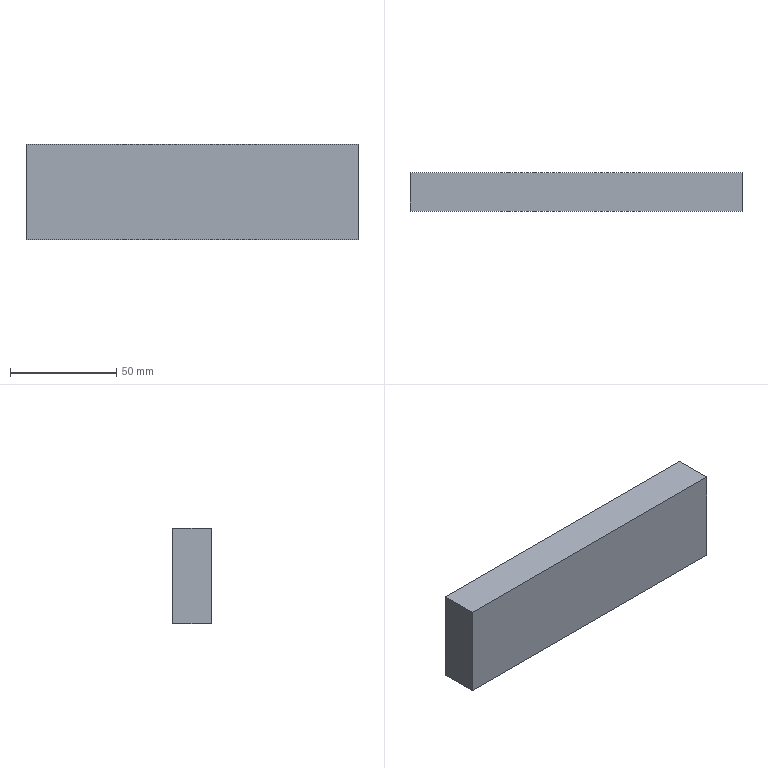NC program | NX | posted with a generic post | part box 156 x 18 x 45 mm
Lines 2243 to 3545 of 3545:
(FLOOR_WALL , TOOL : D4C)
N4424 T03 M6
N4426 G53
N4428 G17 G0 G90 X-18.397 Y-4.1 S3500 M3
N4430 G43 Z19.87 H3
N4432 Z1.825
N4434 G94 G1 Z-0.175 F1500.
N4436 Y-2.
N4438 Y42.
N4440 X-17.1
N4442 Y-2.
N4444 Y-4.1
N4446 Z1.825
N4448 G0 X-18.397 Z1.63
N4450 G1 Z-0.37
N4452 Y-2.
N4454 Y42.
N4456 X-17.1
N4458 Y-2.
N4460 Y-4.1
N4462 Z1.63
N4464 G0 X-18.397 Z1.434
N4466 G1 Z-0.566
N4468 Y-2.
N4470 Y42.
N4472 X-17.1
N4474 Y-2.
N4476 Y-4.1
N4478 Z1.434
N4480 G0 X-18.397 Z1.239
N4482 G1 Z-0.761
N4484 Y-2.
N4486 Y42.
N4488 X-17.1
N4490 Y-2.
N4492 Y-4.1
N4494 Z1.239
N4496 G0 X-18.397 Z1.044
N4498 G1 Z-0.956
N4500 Y-2.
N4502 Y42.
N4504 X-17.1
N4506 Y-2.
N4508 Y-4.1
N4510 Z1.044
N4512 G0 X-18.397 Z0.849
N4514 G1 Z-1.151
N4516 Y-2.
N4518 Y42.
N4520 X-17.1
N4522 Y-2.
N4524 Y-4.1
N4526 Z0.849
N4528 G0 X-18.397 Z0.653
N4530 G1 Z-1.347
N4532 Y-2.
N4534 Y42.
N4536 X-17.1
N4538 Y-2.
N4540 Y-4.1
N4542 Z0.653
N4544 G0 X-18.397 Z0.458
N4546 G1 Z-1.542
N4548 Y-2.
N4550 Y42.
N4552 X-17.1
N4554 Y-2.
N4556 Y-4.1
N4558 Z0.458
N4560 G0 X-18.397 Z0.263
N4562 G1 Z-1.737
N4564 Y-2.
N4566 Y42.
N4568 X-17.1
N4570 Y-2.
N4572 Y-4.1
N4574 Z0.263
N4576 G0 X-18.397 Z0.068
N4578 G1 Z-1.932
N4580 Y-2.
N4582 Y42.
N4584 X-17.1
N4586 Y-2.
N4588 Y-4.1
N4590 Z0.068
N4592 G0 X-18.397 Z-0.128
N4594 G1 Z-2.128
N4596 Y-2.
N4598 Y42.
N4600 X-17.1
N4602 Y-2.
N4604 Y-4.1
N4606 Z-0.128
N4608 G0 X-18.397 Z-0.323
N4610 G1 Z-2.323
N4612 Y-2.
N4614 Y42.
N4616 X-17.1
N4618 Y-2.
N4620 Y-4.1
N4622 Z-0.323
N4624 G0 X-18.397 Z-0.518
N4626 G1 Z-2.518
N4628 Y-2.
N4630 Y42.
N4632 X-17.1
N4634 Y-2.
N4636 Y-4.1
N4638 Z-0.518
N4640 G0 X-18.397 Z-0.713
N4642 G1 Z-2.713
N4644 Y-2.
N4646 Y42.
N4648 X-17.1
N4650 Y-2.
N4652 Y-4.1
N4654 Z-0.713
N4656 G0 X-18.397 Z-0.909
N4658 G1 Z-2.909
N4660 Y-2.
N4662 Y42.
N4664 X-17.1
N4666 Y-2.
N4668 Y-4.1
N4670 Z-0.909
N4672 G0 X-18.397 Z-1.104
N4674 G1 Z-3.104
N4676 Y-2.
N4678 Y42.
N4680 X-17.1
N4682 Y-2.
N4684 Y-4.1
N4686 Z-1.104
N4688 G0 X-18.397 Z-1.299
N4690 G1 Z-3.299
N4692 Y-2.
N4694 Y42.
N4696 X-17.1
N4698 Y-2.
N4700 Y-4.1
N4702 Z-1.299
N4704 G0 X-18.397 Z-1.494
N4706 G1 Z-3.494
N4708 Y-2.
N4710 Y42.
N4712 X-17.1
N4714 Y-2.
N4716 Y-4.1
N4718 Z-1.494
N4720 G0 X-18.397 Z-1.69
N4722 G1 Z-3.69
N4724 Y-2.
N4726 Y42.
N4728 X-17.1
N4730 Y-2.
N4732 Y-4.1
N4734 Z-1.69
N4736 G0 X-18.397 Z-1.885
N4738 G1 Z-3.885
N4740 Y-2.
N4742 Y42.
N4744 X-17.1
N4746 Y-2.
N4748 Y-4.1
N4750 Z-1.885
N4752 G0 X-18.397 Z-2.08
N4754 G1 Z-4.08
N4756 Y-2.
N4758 Y42.
N4760 X-17.1
N4762 Y-2.
N4764 Y-4.1
N4766 Z-2.08
N4768 G0 Z19.87
(PLANAR_MILL_4 , TOOL : D4C)
N4770 X-6.35 Y28.212
N4772 Z0.37
N4774 G1 Y33.264 Z0.357
N4776 X-6.666 Y33.834 Z0.355
N4778 X-7.236 Y34.15 Z0.353
N4780 X-7.764 Z0.352
N4782 X-8.334 Y33.834 Z0.35
N4784 X-8.65 Y33.264 Z0.349
N4786 Y6.736 Z0.279
N4788 X-8.334 Y6.166 Z0.277
N4790 X-7.764 Y5.85 Z0.276
N4792 X-7.236 Z0.274
N4794 X-6.666 Y6.166 Z0.273
N4796 X-6.35 Y6.736 Z0.271
N4798 Y33.264 Z0.201
N4800 X-6.666 Y33.834 Z0.2
N4802 X-7.236 Y34.15 Z0.198
N4804 X-7.764 Z0.197
N4806 X-8.334 Y33.834 Z0.195
N4808 X-8.65 Y33.264 Z0.193
N4810 Y6.736 Z0.124
N4812 X-8.334 Y6.166 Z0.122
N4814 X-7.764 Y5.85 Z0.12
N4816 X-7.236 Z0.119
N4818 X-6.666 Y6.166 Z0.117
N4820 X-6.35 Y6.736 Z0.116
N4822 Y33.264 Z0.046
N4824 X-6.666 Y33.834 Z0.044
N4826 X-7.236 Y34.15 Z0.043
N4828 X-7.764 Z0.041
N4830 X-8.334 Y33.834 Z0.04
N4832 X-8.65 Y33.264 Z0.038
N4834 Y6.736 Z-0.032
N4836 X-8.334 Y6.166 Z-0.033
N4838 X-7.764 Y5.85 Z-0.035
N4840 X-7.236 Z-0.036
N4842 X-6.666 Y6.166 Z-0.038
N4844 X-6.35 Y6.736 Z-0.04
N4846 Y33.264 Z-0.109
N4848 X-6.666 Y33.834 Z-0.111
N4850 X-7.236 Y34.15 Z-0.113
N4852 X-7.764 Z-0.114
N4854 X-8.334 Y33.834 Z-0.116
N4856 X-8.65 Y33.264 Z-0.117
N4858 Y6.736 Z-0.187
N4860 X-8.334 Y6.166 Z-0.189
N4862 X-7.764 Y5.85 Z-0.19
N4864 X-7.236 Z-0.192
N4866 X-6.666 Y6.166 Z-0.193
N4868 X-6.35 Y6.736 Z-0.195
N4870 Y33.264 Z-0.265
N4872 X-6.666 Y33.834 Z-0.266
N4874 X-7.236 Y34.15 Z-0.268
N4876 X-7.764 Z-0.269
N4878 X-8.334 Y33.834 Z-0.271
N4880 X-8.65 Y33.264 Z-0.273
N4882 Y6.736 Z-0.342
N4884 X-8.334 Y6.166 Z-0.344
N4886 X-7.764 Y5.85 Z-0.346
N4888 X-7.236 Z-0.347
N4890 X-6.666 Y6.166 Z-0.349
N4892 X-6.35 Y6.736 Z-0.35
N4894 Y33.264 Z-0.42
N4896 X-6.666 Y33.834 Z-0.422
N4898 X-7.236 Y34.15 Z-0.423
N4900 X-7.764 Z-0.425
N4902 X-8.334 Y33.834 Z-0.426
N4904 X-8.65 Y33.264 Z-0.428
N4906 Y6.736 Z-0.497
N4908 X-8.334 Y6.166 Z-0.499
N4910 X-7.764 Y5.85 Z-0.501
N4912 X-7.236 Z-0.502
N4914 X-6.666 Y6.166 Z-0.504
N4916 X-6.35 Y6.736 Z-0.506
N4918 Y33.264 Z-0.575
N4920 X-6.666 Y33.834 Z-0.577
N4922 X-7.236 Y34.15 Z-0.579
N4924 X-7.764 Z-0.58
N4926 X-8.334 Y33.834 Z-0.582
N4928 X-8.65 Y33.264 Z-0.583
N4930 Y6.736 Z-0.653
N4932 X-8.334 Y6.166 Z-0.655
N4934 X-7.764 Y5.85 Z-0.656
N4936 X-7.236 Z-0.658
N4938 X-6.666 Y6.166 Z-0.659
N4940 X-6.35 Y6.736 Z-0.661
N4942 Y33.264 Z-0.73
N4944 X-6.666 Y33.834 Z-0.732
N4946 X-7.236 Y34.15 Z-0.734
N4948 X-7.764 Z-0.735
N4950 X-8.334 Y33.834 Z-0.737
N4952 X-8.65 Y33.264 Z-0.739
N4954 Y6.736 Z-0.808
N4956 X-8.334 Y6.166 Z-0.81
N4958 X-7.764 Y5.85 Z-0.812
N4960 X-7.236 Z-0.813
N4962 X-6.666 Y6.166 Z-0.815
N4964 X-6.35 Y6.736 Z-0.816
N4966 Y33.264 Z-0.886
N4968 X-6.666 Y33.834 Z-0.887
N4970 X-7.236 Y34.15 Z-0.889
N4972 X-7.764 Z-0.891
N4974 X-8.334 Y33.834 Z-0.892
N4976 X-8.65 Y33.264 Z-0.894
N4978 Y6.736 Z-0.963
N4980 X-8.334 Y6.166 Z-0.965
N4982 X-7.764 Y5.85 Z-0.967
N4984 X-7.236 Z-0.968
N4986 X-6.666 Y6.166 Z-0.97
N4988 X-6.35 Y6.736 Z-0.972
N4990 Y33.264 Z-1.041
N4992 X-6.666 Y33.834 Z-1.043
N4994 X-7.236 Y34.15 Z-1.045
N4996 X-7.764 Z-1.046
N4998 X-8.334 Y33.834 Z-1.048
N5000 X-8.65 Y33.264 Z-1.049
N5002 Y6.736 Z-1.119
N5004 X-8.334 Y6.166 Z-1.12
N5006 X-7.764 Y5.85 Z-1.122
N5008 X-7.236 Z-1.124
N5010 X-6.666 Y6.166 Z-1.125
N5012 X-6.35 Y6.736 Z-1.127
N5014 Y33.264 Z-1.196
N5016 X-6.666 Y33.834 Z-1.198
N5018 X-7.236 Y34.15 Z-1.2
N5020 X-7.764 Z-1.201
N5022 X-8.334 Y33.834 Z-1.203
N5024 X-8.65 Y33.264 Z-1.205
N5026 Y6.736 Z-1.274
N5028 X-8.334 Y6.166 Z-1.276
N5030 X-7.764 Y5.85 Z-1.277
N5032 X-7.236 Z-1.279
N5034 X-6.666 Y6.166 Z-1.281
N5036 X-6.35 Y6.736 Z-1.282
N5038 Y33.264 Z-1.352
N5040 X-6.666 Y33.834 Z-1.353
N5042 X-7.236 Y34.15 Z-1.355
N5044 X-7.764 Z-1.357
N5046 X-8.334 Y33.834 Z-1.358
N5048 X-8.65 Y33.264 Z-1.36
N5050 Y6.736 Z-1.429
N5052 X-8.334 Y6.166 Z-1.431
N5054 X-7.764 Y5.85 Z-1.433
N5056 X-7.236 Z-1.434
N5058 X-6.666 Y6.166 Z-1.436
N5060 X-6.35 Y6.736 Z-1.438
N5062 Y33.264 Z-1.507
N5064 X-6.666 Y33.834 Z-1.509
N5066 X-7.236 Y34.15 Z-1.51
N5068 X-7.764 Z-1.512
N5070 X-8.334 Y33.834 Z-1.514
N5072 X-8.65 Y33.264 Z-1.515
N5074 Y6.736 Z-1.585
N5076 X-8.334 Y6.166 Z-1.586
N5078 X-7.764 Y5.85 Z-1.588
N5080 X-7.236 Z-1.59
N5082 X-6.666 Y6.166 Z-1.591
N5084 X-6.35 Y6.736 Z-1.593
N5086 Y33.264 Z-1.662
N5088 X-6.666 Y33.834 Z-1.664
N5090 X-7.236 Y34.15 Z-1.666
N5092 X-7.764 Z-1.667
N5094 X-8.334 Y33.834 Z-1.669
N5096 X-8.65 Y33.264 Z-1.671
N5098 Y6.736 Z-1.74
N5100 X-8.334 Y6.166 Z-1.742
N5102 X-7.764 Y5.85 Z-1.743
N5104 X-7.236 Z-1.745
N5106 X-6.666 Y6.166 Z-1.747
N5108 X-6.35 Y6.736 Z-1.748
N5110 Y33.264 Z-1.818
N5112 X-6.666 Y33.834 Z-1.819
N5114 X-7.236 Y34.15 Z-1.821
N5116 X-7.764 Z-1.822
N5118 X-8.334 Y33.834 Z-1.824
N5120 X-8.65 Y33.264 Z-1.826
N5122 Y6.736 Z-1.895
N5124 X-8.334 Y6.166 Z-1.897
N5126 X-7.764 Y5.85 Z-1.899
N5128 X-7.236 Z-1.9
N5130 X-6.666 Y6.166 Z-1.902
N5132 X-6.35 Y6.736 Z-1.904
N5134 Y33.264 Z-1.973
N5136 X-6.666 Y33.834 Z-1.975
N5138 X-7.236 Y34.15 Z-1.976
N5140 X-7.764 Z-1.978
N5142 X-8.334 Y33.834 Z-1.98
N5144 X-8.65 Y33.264 Z-1.981
N5146 Y6.736 Z-2.051
N5148 X-8.334 Y6.166 Z-2.052
N5150 X-7.764 Y5.85 Z-2.054
N5152 X-7.236 Z-2.055
N5154 X-6.666 Y6.166 Z-2.057
N5156 X-6.35 Y6.736 Z-2.059
N5158 Y33.264 Z-2.128
N5160 X-6.666 Y33.834 Z-2.13
N5162 X-7.236 Y34.15 Z-2.132
N5164 X-7.764 Z-2.133
N5166 X-8.334 Y33.834 Z-2.135
N5168 X-8.65 Y33.264 Z-2.137
N5170 Y6.736 Z-2.206
N5172 X-8.334 Y6.166 Z-2.208
N5174 X-7.764 Y5.85 Z-2.209
N5176 X-7.236 Z-2.211
N5178 X-6.666 Y6.166 Z-2.212
N5180 X-6.35 Y6.736 Z-2.214
N5182 Y33.264 Z-2.284
N5184 X-6.666 Y33.834 Z-2.285
N5186 X-7.236 Y34.15 Z-2.287
N5188 X-7.764 Z-2.288
N5190 X-8.334 Y33.834 Z-2.29
N5192 X-8.65 Y33.264 Z-2.292
N5194 Y6.736 Z-2.361
N5196 X-8.334 Y6.166 Z-2.363
N5198 X-7.764 Y5.85 Z-2.365
N5200 X-7.236 Z-2.366
N5202 X-6.666 Y6.166 Z-2.368
N5204 X-6.35 Y6.736 Z-2.37
N5206 Y33.264 Z-2.439
N5208 X-6.666 Y33.834 Z-2.441
N5210 X-7.236 Y34.15 Z-2.442
N5212 X-7.764 Z-2.444
N5214 X-8.334 Y33.834 Z-2.445
N5216 X-8.65 Y33.264 Z-2.447
N5218 Y6.736 Z-2.517
N5220 X-8.334 Y6.166 Z-2.518
N5222 X-7.764 Y5.85 Z-2.52
N5224 X-7.236 Z-2.521
N5226 X-6.666 Y6.166 Z-2.523
N5228 X-6.35 Y6.736 Z-2.525
N5230 Y33.264 Z-2.594
N5232 X-6.666 Y33.834 Z-2.596
N5234 X-7.236 Y34.15 Z-2.598
N5236 X-7.764 Z-2.599
N5238 X-8.334 Y33.834 Z-2.601
N5240 X-8.65 Y33.264 Z-2.603
N5242 Y6.736 Z-2.672
N5244 X-8.334 Y6.166 Z-2.674
N5246 X-7.764 Y5.85 Z-2.675
N5248 X-7.236 Z-2.677
N5250 X-6.666 Y6.166 Z-2.678
N5252 X-6.35 Y6.736 Z-2.68
N5254 Y33.264 Z-2.75
N5256 X-6.666 Y33.834 Z-2.751
N5258 X-7.236 Y34.15 Z-2.753
N5260 X-7.764 Z-2.754
N5262 X-8.334 Y33.834 Z-2.756
N5264 X-8.65 Y33.264 Z-2.758
N5266 Y6.736 Z-2.827
N5268 X-8.334 Y6.166 Z-2.829
N5270 X-7.764 Y5.85 Z-2.831
N5272 X-7.236 Z-2.832
N5274 X-6.666 Y6.166 Z-2.834
N5276 X-6.35 Y6.736 Z-2.835
N5278 Y33.264 Z-2.905
N5280 X-6.666 Y33.834 Z-2.907
N5282 X-7.236 Y34.15 Z-2.908
N5284 X-7.764 Z-2.91
N5286 X-8.334 Y33.834 Z-2.911
N5288 X-8.65 Y33.264 Z-2.913
N5290 Y6.736 Z-2.983
N5292 X-8.334 Y6.166 Z-2.984
N5294 X-7.764 Y5.85 Z-2.986
N5296 X-7.236 Z-2.987
N5298 X-6.666 Y6.166 Z-2.989
N5300 X-6.35 Y6.736 Z-2.991
N5302 Y33.264 Z-3.06
N5304 X-6.666 Y33.834 Z-3.062
N5306 X-7.236 Y34.15 Z-3.064
N5308 X-7.764 Z-3.065
N5310 X-8.334 Y33.834 Z-3.067
N5312 X-8.65 Y33.264 Z-3.068
N5314 Y6.736 Z-3.138
N5316 X-8.334 Y6.166 Z-3.14
N5318 X-7.764 Y5.85 Z-3.141
N5320 X-7.236 Z-3.143
N5322 X-6.666 Y6.166 Z-3.144
N5324 X-6.35 Y6.736 Z-3.146
N5326 Y33.264 Z-3.216
N5328 X-6.666 Y33.834 Z-3.217
N5330 X-7.236 Y34.15 Z-3.219
N5332 X-7.764 Z-3.22
N5334 X-8.334 Y33.834 Z-3.222
N5336 X-8.65 Y33.264 Z-3.224
N5338 Y6.736 Z-3.293
N5340 X-8.334 Y6.166 Z-3.295
N5342 X-7.764 Y5.85 Z-3.297
N5344 X-7.236 Z-3.298
N5346 X-6.666 Y6.166 Z-3.3
N5348 X-6.35 Y6.736 Z-3.301
N5350 Y33.264 Z-3.371
N5352 X-6.666 Y33.834 Z-3.373
N5354 X-7.236 Y34.15 Z-3.374
N5356 X-7.764 Z-3.376
N5358 X-8.334 Y33.834 Z-3.377
N5360 X-8.65 Y33.264 Z-3.379
N5362 Y6.736 Z-3.449
N5364 X-8.334 Y6.166 Z-3.45
N5366 X-7.764 Y5.85 Z-3.452
N5368 X-7.236 Z-3.453
N5370 X-6.666 Y6.166 Z-3.455
N5372 X-6.35 Y6.736 Z-3.457
N5374 Y33.264 Z-3.526
N5376 X-6.666 Y33.834 Z-3.528
N5378 X-7.236 Y34.15 Z-3.53
N5380 X-7.764 Z-3.531
N5382 X-8.334 Y33.834 Z-3.533
N5384 X-8.65 Y33.264 Z-3.534
N5386 Y6.736 Z-3.604
N5388 X-8.334 Y6.166 Z-3.606
N5390 X-7.764 Y5.85 Z-3.607
N5392 X-7.236 Z-3.609
N5394 X-6.666 Y6.166 Z-3.61
N5396 X-6.35 Y6.736 Z-3.612
N5398 Y33.264 Z-3.682
N5400 X-6.666 Y33.834 Z-3.683
N5402 X-7.236 Y34.15 Z-3.685
N5404 X-7.764 Z-3.686
N5406 X-8.334 Y33.834 Z-3.688
N5408 X-8.65 Y33.264 Z-3.69
N5410 Y6.736 Z-3.759
N5412 X-8.334 Y6.166 Z-3.761
N5414 X-7.764 Y5.85 Z-3.763
N5416 X-7.236 Z-3.764
N5418 X-6.666 Y6.166 Z-3.766
N5420 X-6.35 Y6.736 Z-3.767
N5422 Y33.264 Z-3.837
N5424 X-6.666 Y33.834 Z-3.839
N5426 X-7.236 Y34.15 Z-3.84
N5428 X-7.764 Z-3.842
N5430 X-8.334 Y33.834 Z-3.843
N5432 X-8.65 Y33.264 Z-3.845
N5434 Y6.736 Z-3.915
N5436 X-8.334 Y6.166 Z-3.916
N5438 X-7.764 Y5.85 Z-3.918
N5440 X-7.236 Z-3.919
N5442 X-6.666 Y6.166 Z-3.921
N5444 X-6.35 Y6.736 Z-3.923
N5446 Y33.264 Z-3.992
N5448 X-6.666 Y33.834 Z-3.994
N5450 X-7.236 Y34.15 Z-3.996
N5452 X-7.764 Z-3.997
N5454 X-8.334 Y33.834 Z-3.999
N5456 X-8.65 Y33.264 Z-4.
N5458 Y6.736 Z-4.07
N5460 X-8.334 Y6.166 Z-4.072
N5462 X-7.764 Y5.85 Z-4.073
N5464 X-7.236 Z-4.075
N5466 X-6.666 Y6.166 Z-4.076
N5468 X-6.35 Y6.736 Z-4.078
N5470 Y33.264 Z-4.147
N5472 X-6.666 Y33.834 Z-4.149
N5474 X-7.236 Y34.15 Z-4.151
N5476 X-7.764 Z-4.152
N5478 X-8.334 Y33.834 Z-4.154
N5480 X-8.65 Y33.264 Z-4.156
N5482 Y6.736 Z-4.225
N5484 X-8.334 Y6.166 Z-4.227
N5486 X-7.764 Y5.85 Z-4.229
N5488 X-7.236 Z-4.23
N5490 X-6.666 Y6.166 Z-4.232
N5492 X-6.35 Y6.736 Z-4.233
N5494 Y33.264 Z-4.303
N5496 X-6.666 Y33.834 Z-4.305
N5498 X-7.236 Y34.15 Z-4.306
N5500 X-7.764 Z-4.308
N5502 X-8.334 Y33.834 Z-4.309
N5504 X-8.65 Y33.264 Z-4.311
N5506 Y6.736 Z-4.38
N5508 X-8.334 Y6.166 Z-4.382
N5510 X-7.764 Y5.85 Z-4.384
N5512 X-7.236 Z-4.385
N5514 X-6.666 Y6.166 Z-4.387
N5516 X-6.35 Y6.736 Z-4.389
N5518 Y33.264 Z-4.458
N5520 X-6.666 Y33.834 Z-4.46
N5522 X-7.236 Y34.15 Z-4.462
N5524 X-7.764 Z-4.463
N5526 X-8.334 Y33.834 Z-4.465
N5528 X-8.65 Y33.264 Z-4.466
N5530 Y6.736 Z-4.536
N5532 X-8.334 Y6.166 Z-4.537
N5534 X-7.764 Y5.85 Z-4.539
N5536 X-7.236 Z-4.541
N5538 X-6.666 Y6.166 Z-4.542
N5540 X-6.35 Y6.736 Z-4.544
N5542 Y33.264 Z-4.613
N5544 X-6.666 Y33.834 Z-4.615
N5546 X-7.236 Y34.15 Z-4.617
N5548 X-7.764 Z-4.618
N5550 X-8.334 Y33.834 Z-4.62
N5552 X-8.65 Y33.264 Z-4.622
N5554 Y6.736 Z-4.691
N5556 X-8.334 Y6.166 Z-4.693
N5558 X-7.764 Y5.85 Z-4.695
N5560 X-7.236 Z-4.696
N5562 X-6.666 Y6.166 Z-4.698
N5564 X-6.35 Y6.736 Z-4.699
N5566 Y33.264 Z-4.769
N5568 X-6.666 Y33.834 Z-4.77
N5570 X-7.236 Y34.15 Z-4.772
N5572 X-7.764 Z-4.774
N5574 X-8.334 Y33.834 Z-4.775
N5576 X-8.65 Y33.264 Z-4.777
N5578 Y6.736 Z-4.846
N5580 X-8.334 Y6.166 Z-4.848
N5582 X-7.764 Y5.85 Z-4.85
N5584 X-7.236 Z-4.851
N5586 X-6.666 Y6.166 Z-4.853
N5588 X-6.35 Y6.736 Z-4.855
N5590 Y33.264 Z-4.924
N5592 X-6.666 Y33.834 Z-4.926
N5594 X-7.236 Y34.15 Z-4.927
N5596 X-7.764 Z-4.929
N5598 X-8.334 Y33.834 Z-4.931
N5600 X-8.65 Y33.264 Z-4.932
N5602 Y6.736 Z-5.002
N5604 X-8.334 Y6.166 Z-5.003
N5606 X-7.764 Y5.85 Z-5.005
N5608 X-7.236 Z-5.007
N5610 X-6.666 Y6.166 Z-5.008
N5612 X-6.35 Y6.736 Z-5.01
N5614 Y33.264 Z-5.079
N5616 X-6.666 Y33.834 Z-5.081
N5618 X-7.236 Y34.15 Z-5.083
N5620 X-7.764 Z-5.084
N5622 X-8.334 Y33.834 Z-5.086
N5624 X-8.65 Y33.264 Z-5.088
N5626 Y6.736 Z-5.157
N5628 X-8.334 Y6.166 Z-5.159
N5630 X-7.764 Y5.85 Z-5.16
N5632 X-7.236 Z-5.162
N5634 X-6.666 Y6.166 Z-5.164
N5636 X-6.35 Y6.736 Z-5.165
N5638 Y33.264 Z-5.235
N5640 X-6.666 Y33.834 Z-5.236
N5642 X-7.236 Y34.15 Z-5.238
N5644 X-7.764 Z-5.24
N5646 X-8.334 Y33.834 Z-5.241
N5648 X-8.65 Y33.264 Z-5.243
N5650 Y6.736 Z-5.312
N5652 X-8.334 Y6.166 Z-5.314
N5654 X-7.764 Y5.85 Z-5.316
N5656 X-7.236 Z-5.317
N5658 X-6.666 Y6.166 Z-5.319
N5660 X-6.35 Y6.736 Z-5.321
N5662 Y33.264 Z-5.39
N5664 X-6.666 Y33.834 Z-5.392
N5666 X-7.236 Y34.15 Z-5.393
N5668 X-7.764 Z-5.395
N5670 X-8.334 Y33.834 Z-5.397
N5672 X-8.65 Y33.264 Z-5.398
N5674 Y6.736 Z-5.468
N5676 X-8.334 Y6.166 Z-5.469
N5678 X-7.764 Y5.85 Z-5.471
N5680 X-7.236 Z-5.472
N5682 X-6.666 Y6.166 Z-5.474
N5684 X-6.35 Y6.736 Z-5.476
N5686 Y33.264 Z-5.545
N5688 X-6.666 Y33.834 Z-5.547
N5690 X-7.236 Y34.15 Z-5.549
N5692 X-7.764 Z-5.55
N5694 X-8.334 Y33.834 Z-5.552
N5696 X-8.65 Y33.264 Z-5.554
N5698 Y6.736 Z-5.623
N5700 X-8.334 Y6.166 Z-5.625
N5702 X-7.764 Y5.85 Z-5.626
N5704 X-7.236 Z-5.628
N5706 X-6.666 Y6.166 Z-5.63
N5708 X-6.35 Y6.736 Z-5.631
N5710 Y33.264 Z-5.701
N5712 X-6.666 Y33.834 Z-5.702
N5714 X-7.236 Y34.15 Z-5.704
N5716 X-7.764 Z-5.705
N5718 X-8.334 Y33.834 Z-5.707
N5720 X-8.65 Y33.264 Z-5.709
N5722 Y6.736 Z-5.778
N5724 X-8.334 Y6.166 Z-5.78
N5726 X-7.764 Y5.85 Z-5.782
N5728 X-7.236 Z-5.783
N5730 X-6.666 Y6.166 Z-5.785
N5732 X-6.35 Y6.736 Z-5.787
N5734 Y33.264 Z-5.856
N5736 X-6.666 Y33.834 Z-5.858
N5738 X-7.236 Y34.15 Z-5.859
N5740 X-7.764 Z-5.861
N5742 X-8.334 Y33.834 Z-5.863
N5744 X-8.65 Y33.264 Z-5.864
N5746 Y6.736 Z-5.934
N5748 X-8.334 Y6.166 Z-5.935
N5750 X-7.764 Y5.85 Z-5.937
N5752 X-7.236 Z-5.938
N5754 X-6.666 Y6.166 Z-5.94
N5756 X-6.35 Y6.736 Z-5.942
N5758 Y33.264 Z-6.011
N5760 X-6.666 Y33.834 Z-6.013
N5762 X-7.236 Y34.15 Z-6.015
N5764 X-7.764 Z-6.016
N5766 X-8.334 Y33.834 Z-6.018
N5768 X-8.65 Y33.264 Z-6.02
N5770 Y6.736 Z-6.089
N5772 X-8.334 Y6.166 Z-6.091
N5774 X-7.764 Y5.85 Z-6.092
N5776 X-7.236 Z-6.094
N5778 X-6.666 Y6.166 Z-6.095
N5780 X-6.35 Y6.736 Z-6.097
N5782 Y33.264 Z-6.167
N5784 X-6.666 Y33.834 Z-6.168
N5786 X-7.236 Y34.15 Z-6.17
N5788 X-7.764 Z-6.171
N5790 X-8.334 Y33.834 Z-6.173
N5792 X-8.65 Y33.264 Z-6.175
N5794 Y6.736 Z-6.244
N5796 X-8.334 Y6.166 Z-6.246
N5798 X-7.764 Y5.85 Z-6.248
N5800 X-7.236 Z-6.249
N5802 X-6.666 Y6.166 Z-6.251
N5804 X-6.35 Y6.736 Z-6.253
N5806 Y33.264 Z-6.322
N5808 X-6.666 Y33.834 Z-6.324
N5810 X-7.236 Y34.15 Z-6.325
N5812 X-7.764 Z-6.327
N5814 X-8.334 Y33.834 Z-6.328
N5816 X-8.65 Y33.264 Z-6.33
N5818 Y6.736 Z-6.4
N5820 X-8.334 Y6.166 Z-6.401
N5822 X-7.764 Y5.85 Z-6.403
N5824 X-7.236 Z-6.404
N5826 X-6.666 Y6.166 Z-6.406
N5828 X-6.35 Y6.736 Z-6.408
N5830 Y33.264 Z-6.477
N5832 X-6.666 Y33.834 Z-6.479
N5834 X-7.236 Y34.15 Z-6.481
N5836 X-7.764 Z-6.482
N5838 X-8.334 Y33.834 Z-6.484
N5840 X-8.65 Y33.264 Z-6.485
N5842 Y6.736 Z-6.555
N5844 X-8.334 Y6.166 Z-6.557
N5846 X-7.764 Y5.85 Z-6.558
N5848 X-7.236 Z-6.56
N5850 X-6.666 Y6.166 Z-6.561
N5852 X-6.35 Y6.736 Z-6.563
N5854 Y33.264 Z-6.633
N5856 X-6.666 Y33.834 Z-6.634
N5858 X-7.236 Y34.15 Z-6.636
N5860 X-7.764 Z-6.637
N5862 X-8.334 Y33.834 Z-6.639
N5864 X-8.65 Y33.264 Z-6.641
N5866 Y6.736 Z-6.71
N5868 X-8.334 Y6.166 Z-6.712
N5870 X-7.764 Y5.85 Z-6.714
N5872 X-7.236 Z-6.715
N5874 X-6.666 Y6.166 Z-6.717
N5876 X-6.35 Y6.736 Z-6.718
N5878 Y33.264 Z-6.788
N5880 X-6.666 Y33.834 Z-6.79
N5882 X-7.236 Y34.15 Z-6.791
N5884 X-7.764 Z-6.793
N5886 X-8.334 Y33.834 Z-6.794
N5888 X-8.65 Y33.264 Z-6.796
N5890 Y6.736 Z-6.866
N5892 X-8.334 Y6.166 Z-6.867
N5894 X-7.764 Y5.85 Z-6.869
N5896 X-7.236 Z-6.87
N5898 X-6.666 Y6.166 Z-6.872
N5900 X-6.35 Y6.736 Z-6.874
N5902 Y33.264 Z-6.943
N5904 X-6.666 Y33.834 Z-6.945
N5906 X-7.236 Y34.15 Z-6.947
N5908 X-7.764 Z-6.948
N5910 X-8.334 Y33.834 Z-6.95
N5912 X-8.65 Y33.264 Z-6.951
N5914 Y6.736 Z-7.021
N5916 X-8.334 Y6.166 Z-7.023
N5918 X-7.764 Y5.85 Z-7.024
N5920 X-7.236 Z-7.026
N5922 X-6.666 Y6.166 Z-7.027
N5924 X-6.35 Y6.736 Z-7.029
N5926 Y33.264 Z-7.099
N5928 X-6.666 Y33.834 Z-7.1
N5930 X-7.236 Y34.15 Z-7.102
N5932 X-7.764 Z-7.103
N5934 X-8.334 Y33.834 Z-7.105
N5936 X-8.65 Y33.264 Z-7.107
N5938 Y6.736 Z-7.176
N5940 X-8.334 Y6.166 Z-7.178
N5942 X-7.764 Y5.85 Z-7.18
N5944 X-7.236 Z-7.181
N5946 X-6.666 Y6.166 Z-7.183
N5948 X-6.35 Y6.736 Z-7.184
N5950 Y33.264 Z-7.254
N5952 X-6.666 Y33.834 Z-7.256
N5954 X-7.236 Y34.15 Z-7.257
N5956 X-7.764 Z-7.259
N5958 X-8.334 Y33.834 Z-7.26
N5960 X-8.65 Y33.264 Z-7.262
N5962 Y6.736 Z-7.332
N5964 X-8.334 Y6.166 Z-7.333
N5966 X-7.764 Y5.85 Z-7.335
N5968 X-7.236 Z-7.336
N5970 X-6.666 Y6.166 Z-7.338
N5972 X-6.35 Y6.736 Z-7.34
N5974 Y33.264 Z-7.409
N5976 X-6.666 Y33.834 Z-7.411
N5978 X-7.236 Y34.15 Z-7.413
N5980 X-7.764 Z-7.414
N5982 X-8.334 Y33.834 Z-7.416
N5984 X-8.65 Y33.264 Z-7.417
N5986 Y6.736 Z-7.487
N5988 X-8.334 Y6.166 Z-7.489
N5990 X-7.764 Y5.85 Z-7.49
N5992 X-7.236 Z-7.492
N5994 X-6.666 Y6.166 Z-7.493
N5996 X-6.35 Y6.736 Z-7.495
N5998 Y33.264 Z-7.565
N6000 X-6.666 Y33.834 Z-7.566
N6002 X-7.236 Y34.15 Z-7.568
N6004 X-7.764 Z-7.569
N6006 X-8.334 Y33.834 Z-7.571
N6008 X-8.65 Y33.264 Z-7.573
N6010 Y6.736 Z-7.642
N6012 X-8.334 Y6.166 Z-7.644
N6014 X-7.764 Y5.85 Z-7.646
N6016 X-7.236 Z-7.647
N6018 X-6.666 Y6.166 Z-7.649
N6020 X-6.35 Y6.736 Z-7.65
N6022 Y33.264 Z-7.72
N6024 X-6.666 Y33.834 Z-7.722
N6026 X-7.236 Y34.15 Z-7.723
N6028 X-7.764 Z-7.725
N6030 X-8.334 Y33.834 Z-7.726
N6032 X-8.65 Y33.264 Z-7.728
N6034 Y6.736 Z-7.797
N6036 X-8.334 Y6.166 Z-7.799
N6038 X-7.764 Y5.85 Z-7.801
N6040 X-7.236 Z-7.802
N6042 X-6.666 Y6.166 Z-7.804
N6044 X-6.35 Y6.736 Z-7.806
N6046 Y33.264 Z-7.875
N6048 X-6.666 Y33.834 Z-7.877
N6050 X-7.236 Y34.15 Z-7.879
N6052 X-7.764 Z-7.88
N6054 X-8.334 Y33.834 Z-7.882
N6056 X-8.65 Y33.264 Z-7.883
N6058 Y6.736 Z-7.953
N6060 X-8.334 Y6.166 Z-7.955
N6062 X-7.764 Y5.85 Z-7.956
N6064 X-7.236 Z-7.958
N6066 X-6.666 Y6.166 Z-7.959
N6068 X-6.35 Y6.736 Z-7.961
N6070 Y33.264 Z-8.03
N6072 X-6.666 Y33.834 Z-8.032
N6074 X-7.236 Y34.15 Z-8.034
N6076 X-7.764 Z-8.035
N6078 X-8.334 Y33.834 Z-8.037
N6080 X-8.65 Y33.264 Z-8.039
N6082 Y6.736 Z-8.108
N6084 X-8.334 Y6.166 Z-8.11
N6086 X-7.764 Y5.85 Z-8.112
N6088 X-7.236 Z-8.113
N6090 X-6.666 Y6.166 Z-8.115
N6092 X-6.35 Y6.736 Z-8.116
N6094 Y33.264 Z-8.186
N6096 X-6.666 Y33.834 Z-8.187
N6098 X-7.236 Y34.15 Z-8.189
N6100 X-7.764 Z-8.191
N6102 X-8.334 Y33.834 Z-8.192
N6104 X-8.65 Y33.264 Z-8.194
N6106 Y6.736 Z-8.263
N6108 X-8.334 Y6.166 Z-8.265
N6110 X-7.764 Y5.85 Z-8.267
N6112 X-7.236 Z-8.268
N6114 X-6.666 Y6.166 Z-8.27
N6116 X-6.35 Y6.736 Z-8.272
N6118 Y33.264 Z-8.341
N6120 X-6.666 Y33.834 Z-8.343
N6122 X-7.236 Y34.15 Z-8.345
N6124 X-7.764 Z-8.346
N6126 X-8.334 Y33.834 Z-8.348
N6128 X-8.65 Y33.264 Z-8.349
N6130 Y6.736 Z-8.419
N6132 X-8.334 Y6.166 Z-8.42
N6134 X-7.764 Y5.85 Z-8.422
N6136 X-7.236 Z-8.424
N6138 X-6.666 Y6.166 Z-8.425
N6140 X-6.35 Y6.736 Z-8.427
N6142 Y33.264 Z-8.496
N6144 X-6.666 Y33.834 Z-8.498
N6146 X-7.236 Y34.15 Z-8.5
N6148 X-7.764 Z-8.501
N6150 X-8.334 Y33.834 Z-8.503
N6152 X-8.65 Y33.264 Z-8.505
N6154 Y6.736 Z-8.574
N6156 X-8.334 Y6.166 Z-8.576
N6158 X-7.764 Y5.85 Z-8.577
N6160 X-7.236 Z-8.579
N6162 X-6.666 Y6.166 Z-8.581
N6164 X-6.35 Y6.736 Z-8.582
N6166 Y33.264 Z-8.652
N6168 X-6.666 Y33.834 Z-8.653
N6170 X-7.236 Y34.15 Z-8.655
N6172 X-7.764 Z-8.657
N6174 X-8.334 Y33.834 Z-8.658
N6176 X-8.65 Y33.264 Z-8.66
N6178 Y6.736 Z-8.729
N6180 X-8.334 Y6.166 Z-8.731
N6182 X-7.764 Y5.85 Z-8.733
N6184 X-7.236 Z-8.734
N6186 X-6.666 Y6.166 Z-8.736
N6188 X-6.35 Y6.736 Z-8.738
N6190 Y33.264 Z-8.807
N6192 X-6.666 Y33.834 Z-8.809
N6194 X-7.236 Y34.15 Z-8.81
N6196 X-7.764 Z-8.812
N6198 X-8.334 Y33.834 Z-8.814
N6200 X-8.65 Y33.264 Z-8.815
N6202 Y6.736 Z-8.885
N6204 X-8.334 Y6.166 Z-8.886
N6206 X-7.764 Y5.85 Z-8.888
N6208 X-7.236 Z-8.89
N6210 X-6.666 Y6.166 Z-8.891
N6212 X-6.35 Y6.736 Z-8.893
N6214 Y33.264 Z-8.962
N6216 X-6.666 Y33.834 Z-8.964
N6218 X-7.236 Y34.15 Z-8.966
N6220 X-7.764 Z-8.967
N6222 X-8.334 Y33.834 Z-8.969
N6224 X-8.65 Y33.264 Z-8.971
N6226 Y6.736 Z-9.04
N6228 X-8.334 Y6.166 Z-9.042
N6230 X-7.764 Y5.85 Z-9.043
N6232 X-7.236 Z-9.045
N6234 X-6.666 Y6.166 Z-9.047
N6236 X-6.35 Y6.736 Z-9.048
N6238 Y33.264 Z-9.118
N6240 X-6.666 Y33.834 Z-9.119
N6242 X-7.236 Y34.15 Z-9.121
N6244 X-7.764 Z-9.122
N6246 X-8.334 Y33.834 Z-9.124
N6248 X-8.65 Y33.264 Z-9.126
N6250 Y6.736 Z-9.195
N6252 X-8.334 Y6.166 Z-9.197
N6254 X-7.764 Y5.85 Z-9.199
N6256 X-7.236 Z-9.2
N6258 X-6.666 Y6.166 Z-9.202
N6260 X-6.35 Y6.736 Z-9.204
N6262 Y33.264 Z-9.273
N6264 X-6.666 Y33.834 Z-9.275
N6266 X-7.236 Y34.15 Z-9.276
N6268 X-7.764 Z-9.278
N6270 X-8.334 Y33.834 Z-9.28
N6272 X-8.65 Y33.264 Z-9.281
N6274 Y6.736 Z-9.351
N6276 X-8.334 Y6.166 Z-9.352
N6278 X-7.764 Y5.85 Z-9.354
N6280 X-7.236 Z-9.355
N6282 X-6.666 Y6.166 Z-9.357
N6284 X-6.35 Y6.736 Z-9.359
N6286 Y33.264 Z-9.428
N6288 X-6.666 Y33.834 Z-9.43
N6290 X-7.236 Y34.15 Z-9.432
N6292 X-7.764 Z-9.433
N6294 X-8.334 Y33.834 Z-9.435
N6296 X-8.65 Y33.264 Z-9.437
N6298 Y6.736 Z-9.506
N6300 X-8.334 Y6.166 Z-9.508
N6302 X-7.764 Y5.85 Z-9.509
N6304 X-7.236 Z-9.511
N6306 X-6.666 Y6.166 Z-9.513
N6308 X-6.35 Y6.736 Z-9.514
N6310 Y33.264 Z-9.584
N6312 X-6.666 Y33.834 Z-9.585
N6314 X-7.236 Y34.15 Z-9.587
N6316 X-7.764 Z-9.588
N6318 X-8.334 Y33.834 Z-9.59
N6320 X-8.65 Y33.264 Z-9.592
N6322 Y6.736 Z-9.661
N6324 X-8.334 Y6.166 Z-9.663
N6326 X-7.764 Y5.85 Z-9.665
N6328 X-7.236 Z-9.666
N6330 X-6.666 Y6.166 Z-9.668
N6332 X-6.35 Y6.736 Z-9.67
N6334 Y33.264 Z-9.739
N6336 X-6.666 Y33.834 Z-9.741
N6338 X-7.236 Y34.15 Z-9.742
N6340 X-7.764 Z-9.744
N6342 X-8.334 Y33.834 Z-9.745
N6344 X-8.65 Y33.264 Z-9.747
N6346 Y6.736 Z-9.817
N6348 X-8.334 Y6.166 Z-9.818
N6350 X-7.764 Y5.85 Z-9.82
N6352 X-7.236 Z-9.821
N6354 X-6.666 Y6.166 Z-9.823
N6356 X-6.35 Y6.736 Z-9.825
N6358 Y33.264 Z-9.894
N6360 X-6.666 Y33.834 Z-9.896
N6362 X-7.236 Y34.15 Z-9.898
N6364 X-7.764 Z-9.899
N6366 X-8.334 Y33.834 Z-9.901
N6368 X-8.65 Y33.264 Z-9.903
N6370 Y6.736 Z-9.972
N6372 X-8.334 Y6.166 Z-9.974
N6374 X-7.764 Y5.85 Z-9.975
N6376 X-7.236 Z-9.977
N6378 X-6.666 Y6.166 Z-9.978
N6380 X-6.35 Y6.736 Z-9.98
N6382 Y33.264 Z-10.05
N6384 X-6.666 Y33.834 Z-10.051
N6386 X-7.236 Y34.15 Z-10.053
N6388 X-7.764 Z-10.054
N6390 X-8.334 Y33.834 Z-10.056
N6392 X-8.65 Y33.264 Z-10.058
N6394 Y6.736 Z-10.127
N6396 X-8.334 Y6.166 Z-10.129
N6398 X-7.764 Y5.85 Z-10.131
N6400 X-7.236 Z-10.132
N6402 X-6.666 Y6.166 Z-10.134
N6404 X-6.35 Y6.736 Z-10.135
N6406 Y33.264 Z-10.205
N6408 X-6.666 Y33.834 Z-10.207
N6410 X-7.236 Y34.15 Z-10.208
N6412 X-7.764 Z-10.21
N6414 X-8.334 Y33.834 Z-10.211
N6416 X-8.65 Y33.264 Z-10.213
N6418 Y6.736 Z-10.283
N6420 X-8.334 Y6.166 Z-10.284
N6422 X-7.764 Y5.85 Z-10.286
N6424 X-7.236 Z-10.287
N6426 X-6.666 Y6.166 Z-10.289
N6428 X-6.35 Y6.736 Z-10.291
N6430 Y33.264 Z-10.36
N6432 X-6.666 Y33.834 Z-10.362
N6434 X-7.236 Y34.15 Z-10.364
N6436 X-7.764 Z-10.365
N6438 X-8.334 Y33.834 Z-10.367
N6440 X-8.65 Y33.264 Z-10.368
N6442 Y6.736 Z-10.438
N6444 X-8.334 Y6.166 Z-10.44
N6446 X-7.764 Y5.85 Z-10.441
N6448 X-7.236 Z-10.443
N6450 X-6.666 Y6.166 Z-10.444
N6452 X-6.35 Y6.736 Z-10.446
N6454 Y33.264 Z-10.516
N6456 X-6.666 Y33.834 Z-10.517
N6458 X-7.236 Y34.15 Z-10.519
N6460 X-7.764 Z-10.52
N6462 X-8.334 Y33.834 Z-10.522
N6464 X-8.65 Y33.264 Z-10.524
N6466 Y6.736 Z-10.593
N6468 X-8.334 Y6.166 Z-10.595
N6470 X-7.764 Y5.85 Z-10.597
N6472 X-7.236 Z-10.598
N6474 X-6.666 Y6.166 Z-10.6
N6476 X-6.35 Y6.736 Z-10.601
N6478 Y33.264 Z-10.671
N6480 X-6.666 Y33.834 Z-10.673
N6482 X-7.236 Y34.15 Z-10.674
N6484 X-7.764 Z-10.676
N6486 X-8.334 Y33.834 Z-10.677
N6488 X-8.65 Y33.264 Z-10.679
N6490 Y6.736 Z-10.749
N6492 X-8.334 Y6.166 Z-10.75
N6494 X-7.764 Y5.85 Z-10.752
N6496 X-7.236 Z-10.753
N6498 X-6.666 Y6.166 Z-10.755
N6500 X-6.35 Y6.736 Z-10.757
N6502 Y33.264 Z-10.826
N6504 X-6.666 Y33.834 Z-10.828
N6506 X-7.236 Y34.15 Z-10.83
N6508 X-7.764 Z-10.831
N6510 X-8.334 Y33.834 Z-10.833
N6512 X-8.65 Y33.264 Z-10.834
N6514 Y6.736 Z-10.904
N6516 X-8.334 Y6.166 Z-10.906
N6518 X-7.764 Y5.85 Z-10.907
N6520 X-7.236 Z-10.909
N6522 X-6.666 Y6.166 Z-10.91
N6524 X-6.35 Y6.736 Z-10.912
N6526 Y33.264 Z-10.982
N6528 X-6.666 Y33.834 Z-10.983
N6530 X-7.236 Y34.15 Z-10.985
N6532 X-7.764 Z-10.986
N6534 X-8.334 Y33.834 Z-10.988
N6536 X-8.65 Y33.264 Z-10.99
N6538 Y6.736 Z-11.059
N6540 X-8.334 Y6.166 Z-11.061
N6542 X-7.764 Y5.85 Z-11.063
N6544 X-7.236 Z-11.064
N6546 X-6.666 Y6.166 Z-11.066
N6548 X-6.35 Y6.736 Z-11.067
N6550 Y33.264 Z-11.137
N6552 X-6.666 Y33.834 Z-11.139
N6554 X-7.236 Y34.15 Z-11.14
N6556 X-7.764 Z-11.142
N6558 X-8.334 Y33.834 Z-11.143
N6560 X-8.65 Y33.264 Z-11.145
N6562 Y6.736 Z-11.215
N6564 X-8.334 Y6.166 Z-11.216
N6566 X-7.764 Y5.85 Z-11.218
N6568 X-7.236 Z-11.219
N6570 X-6.666 Y6.166 Z-11.221
N6572 X-6.35 Y6.736 Z-11.223
N6574 Y33.264 Z-11.292
N6576 X-6.666 Y33.834 Z-11.294
N6578 X-7.236 Y34.15 Z-11.296
N6580 X-7.764 Z-11.297
N6582 X-8.334 Y33.834 Z-11.299
N6584 X-8.65 Y33.264 Z-11.3
N6586 Y6.736 Z-11.37
N6588 X-8.334 Y6.166 Z-11.372
N6590 X-7.764 Y5.85 Z-11.373
N6592 X-7.236 Z-11.375
N6594 X-6.666 Y6.166 Z-11.376
N6596 X-6.35 Y6.736 Z-11.378
N6598 Y33.264 Z-11.447
N6600 X-6.666 Y33.834 Z-11.449
N6602 X-7.236 Y34.15 Z-11.451
N6604 X-7.764 Z-11.452
N6606 X-8.334 Y33.834 Z-11.454
N6608 X-8.65 Y33.264 Z-11.456
N6610 Y6.736 Z-11.525
N6612 X-8.334 Y6.166 Z-11.527
N6614 X-7.764 Y5.85 Z-11.529
N6616 X-7.236 Z-11.53
N6618 X-6.666 Y6.166 Z-11.532
N6620 X-6.35 Y6.736 Z-11.533
N6622 Y33.264 Z-11.603
N6624 X-6.666 Y33.834 Z-11.605
N6626 X-7.236 Y34.15 Z-11.606
N6628 X-7.764 Z-11.608
N6630 X-8.334 Y33.834 Z-11.609
N6632 X-8.65 Y33.264 Z-11.611
N6634 Y6.736 Z-11.68
N6636 X-8.334 Y6.166 Z-11.682
N6638 X-7.764 Y5.85 Z-11.684
N6640 X-7.236 Z-11.685
N6642 X-6.666 Y6.166 Z-11.687
N6644 X-6.35 Y6.736 Z-11.689
N6646 Y33.264 Z-11.758
N6648 X-6.666 Y33.834 Z-11.76
N6650 X-7.236 Y34.15 Z-11.762
N6652 X-7.764 Z-11.763
N6654 X-8.334 Y33.834 Z-11.765
N6656 X-8.65 Y33.264 Z-11.766
N6658 Y6.736 Z-11.836
N6660 X-8.334 Y6.166 Z-11.837
N6662 X-7.764 Y5.85 Z-11.839
N6664 X-7.236 Z-11.841
N6666 X-6.666 Y6.166 Z-11.842
N6668 X-6.35 Y6.736 Z-11.844
N6670 Y33.264 Z-11.913
N6672 X-6.666 Y33.834 Z-11.915
N6674 X-7.236 Y34.15 Z-11.917
N6676 X-7.764 Z-11.918
N6678 X-8.334 Y33.834 Z-11.92
N6680 X-8.65 Y33.264 Z-11.922
N6682 Y6.736 Z-11.991
N6684 X-8.334 Y6.166 Z-11.993
N6686 X-7.764 Y5.85 Z-11.995
N6688 X-7.236 Z-11.996
N6690 X-6.666 Y6.166 Z-11.998
N6692 X-6.35 Y6.736 Z-11.999
N6694 Y33.264 Z-12.069
N6696 X-6.666 Y33.834 Z-12.07
N6698 X-7.236 Y34.15 Z-12.072
N6700 X-7.764 Z-12.074
N6702 X-8.334 Y33.834 Z-12.075
N6704 X-8.65 Y33.264 Z-12.077
N6706 Y6.736 Z-12.146
N6708 X-8.334 Y6.166 Z-12.148
N6710 X-7.764 Y5.85 Z-12.15
N6712 X-7.236 Z-12.151
N6714 X-6.666 Y6.166 Z-12.153
N6716 X-6.35 Y6.736 Z-12.155
N6718 Y33.264 Z-12.224
N6720 X-6.666 Y33.834 Z-12.226
N6722 X-7.236 Y34.15 Z-12.228
N6724 X-7.764 Z-12.229
N6726 X-8.334 Y33.834 Z-12.231
N6728 X-8.65 Y33.264 Z-12.232
N6730 Y6.736 Z-12.302
N6732 X-8.334 Y6.166 Z-12.303
N6734 X-7.764 Y5.85 Z-12.305
N6736 X-7.236 Z-12.307
N6738 X-6.666 Y6.166 Z-12.308
N6740 X-6.35 Y6.736 Z-12.31
N6742 Y33.264 Z-12.379
N6744 X-6.666 Y33.834 Z-12.381
N6746 X-7.236 Y34.15 Z-12.383
N6748 X-7.764 Z-12.384
N6750 X-8.334 Y33.834 Z-12.386
N6752 X-8.65 Y33.264 Z-12.388
N6754 Y6.736 Z-12.457
N6756 X-8.334 Y6.166 Z-12.459
N6758 X-7.764 Y5.85 Z-12.46
N6760 X-7.236 Z-12.462
N6762 X-6.666 Y6.166 Z-12.464
N6764 X-6.35 Y6.736 Z-12.465
N6766 Y20. Z-12.5
N6768 Y33.
N6770 G3 X-7.5 Y34.15 R1.15
N6772 X-8.65 Y33. R1.15
N6774 G1 Y7.
N6776 G3 X-7.5 Y5.85 R1.15
N6778 X-6.35 Y7. R1.15
N6780 G1 Y20.
N6782 Z-12.
N6784 G0 Z19.87
N6786 M5
(FLOOR_WALL_COPY , TOOL : D4J)
N6788 T04 M6
N6790 G53
N6792 G17 G0 G90 X-18.497 Y-4. S3000 M3
N6794 G43 Z19.87 H4
N6796 Z-2.18
N6798 G94 G1 Z-4.18 F400.
N6800 Y-2.
N6802 Y42.
N6804 X-17.
N6806 Y-2.
N6808 Y-4.
N6810 Z-2.18
N6812 G0 Z19.87
(PLANAR_MILL_4_COPY , TOOL : D4J)
N6814 X-8.053 Y20.465 S3500
N6816 Z-10.5
N6818 G1 Z-12.5 F1500.
N6820 G41 X-8.25 Y20.5 D4
N6822 G3 X-8.75 Y20. R0.5
N6824 G1 Y7.
N6826 G3 X-7.5 Y5.75 R1.25
N6828 X-6.25 Y7. R1.25
N6830 G1 Y33.
N6832 G3 X-7.5 Y34.25 R1.25
N6834 X-8.75 Y33. R1.25
N6836 G1 Y20.
N6838 G3 X-8.25 Y19.5 R0.5
N6840 G40
N6842 G1 X-8.053 Y19.535
N6844 Y20.465
N6846 G41 X-8.25 Y20.5
N6848 G3 X-8.75 Y20. R0.5
N6850 G1 Y7.
N6852 G3 X-7.5 Y5.75 R1.25
N6854 X-6.25 Y7. R1.25
N6856 G1 Y33.
N6858 G3 X-7.5 Y34.25 R1.25
N6860 X-8.75 Y33. R1.25
N6862 G1 Y20.
N6864 G3 X-8.25 Y19.5 R0.5
N6866 G40
N6868 G1 X-8.053 Y19.535
N6870 Z-10.5
N6872 G0 Z19.87
N6874 M5
(PLANAR_MILL_5_COPY_1 , TOOL : D4DJ)
N6876 T05 M6
N6878 G53
N6880 G17 G0 G90 X-152.121 Y9.707 S3000 M3
N6882 G43 Z19.87 H5
N6884 Z1.
N6886 G94 G1 Z-1. F1000.
N6888 G3 X-150.707 Y9.707 R1.
N6890 G1 X-149.707 Y10.707
N6892 G2 X-149. Y11. R1.
N6894 G1 X-26.
N6896 G3 X-24. Y13. R2.
N6898 G1 Y39.
N6900 G2 X-23.707 Y39.707 R1.
N6902 G1 X-22.707 Y40.707
N6904 G2 X-22. Y41. R1.
N6906 G1 X-20.5
N6908 G2 X-19.5 Y40. R1.
N6910 G1 Y0.
N6912 G3 X-18.5 Y-1. R1.
N6914 G1 Z1.
N6916 G0 Z19.87
(PLANAR_MILL_5_COPY , TOOL : D4DJ)
N6918 X-6.25 Y32.
N6920 Z0.87
N6922 G1 Z-1.13
N6924 G3 X-5.25 Y33. R1.
N6926 X-7.5 Y35.25 R2.25
N6928 X-9.75 Y33. R2.25
N6930 G1 Y7.
N6932 G3 X-7.5 Y4.75 R2.25
N6934 X-5.25 Y7. R2.25
N6936 G1 Y33.
N6938 G3 X-6.25 Y34. R1.
N6940 G1 X-6.75
N6942 Z0.87
N6944 G0 Z19.87
(PLANAR_MILL_5 , TOOL : D4DJ)
N6946 X1.029 Y-0.615
N6948 Z1.
N6950 G1 Z-1.
N6952 G3 X-0.385 Y-0.615 R1.
N6954 G2 X-1. Y-0.87 R0.87
N6956 G1 X-15.
N6958 G2 X-15.87 Y0. R0.87
N6960 G1 Y40.
N6962 G2 X-15. Y40.87 R0.87
N6964 G1 X-1.
N6966 G2 X-0.385 Y40.615 R0.87
N6968 G1 X0.615 Y39.615
N6970 G2 X0.87 Y39. R0.87
N6972 G1 Y1.
N6974 G2 X0.615 Y0.385 R0.87
N6976 G1 X-0.385 Y-0.615
N6978 G3 X-0.385 Y-2.029 R1.
N6980 G1 Z1.
N6982 G0 Z19.87
N6984 M5
N6986 M2